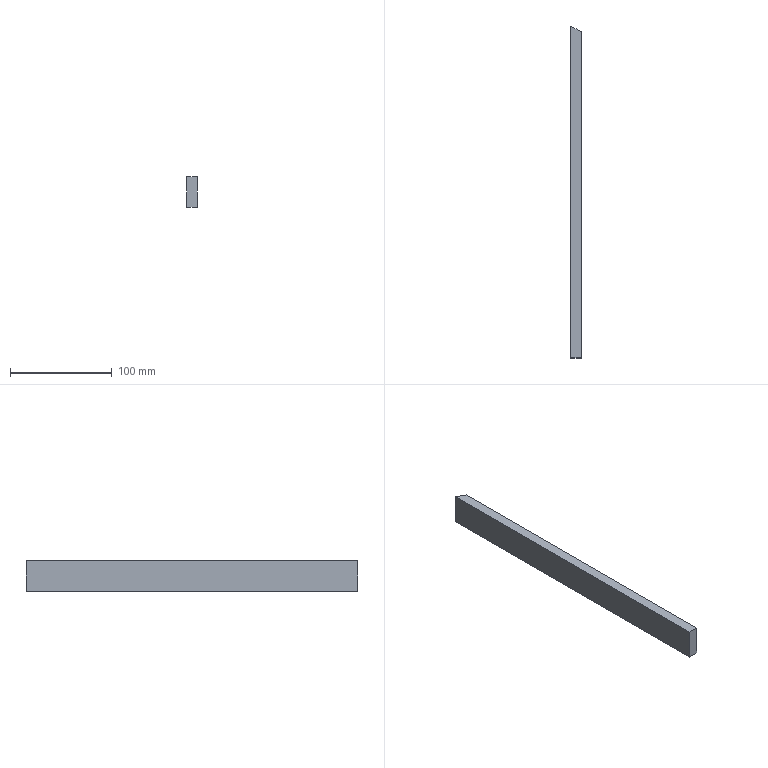Part | NX | features solid 2 | 1 solid | 6 faces | box 10 x 326.105 x 30 mm | volume 96966 mm3 | plane 6
STEP:
#1=CARTESIAN_POINT('',(675.,-588.785,-135.));
#2=VERTEX_POINT('',#1);
#3=CARTESIAN_POINT('',(675.,-588.785,-105.));
#4=VERTEX_POINT('',#3);
#5=CARTESIAN_POINT('',(675.,-588.785,-135.));
#6=DIRECTION('',(0.,0.,-1.));
#7=VECTOR('',#6,1000.);
#8=LINE('',#5,#7);
#9=EDGE_CURVE('',#2,#4,#8,.F.);
#10=ORIENTED_EDGE('',*,*,#9,.F.);
#11=CARTESIAN_POINT('',(675.,-268.453,-135.));
#12=VERTEX_POINT('',#11);
#13=CARTESIAN_POINT('',(675.,-568.785,-135.));
#14=DIRECTION('',(0.,1.,0.));
#15=VECTOR('',#14,1000.);
#16=LINE('',#13,#15);
#17=EDGE_CURVE('',#2,#12,#16,.T.);
#18=ORIENTED_EDGE('',*,*,#17,.T.);
#19=CARTESIAN_POINT('',(675.,-268.453,-105.));
#20=VERTEX_POINT('',#19);
#21=CARTESIAN_POINT('',(675.,-268.453,-135.));
#22=DIRECTION('',(0.,0.,1.));
#23=VECTOR('',#22,1000.);
#24=LINE('',#21,#23);
#25=EDGE_CURVE('',#20,#12,#24,.F.);
#26=ORIENTED_EDGE('',*,*,#25,.F.);
#27=CARTESIAN_POINT('',(675.,-568.785,-105.));
#28=DIRECTION('',(0.,1.,0.));
#29=VECTOR('',#28,1000.);
#30=LINE('',#27,#29);
#31=EDGE_CURVE('',#4,#20,#30,.T.);
#32=ORIENTED_EDGE('',*,*,#31,.F.);
#33=EDGE_LOOP('',(#10,#18,#26,#32));
#34=FACE_BOUND('',#33,.T.);
#35=CARTESIAN_POINT('',(675.,-568.785,-135.));
#36=DIRECTION('',(1.,0.,0.));
#37=DIRECTION('',(0.,0.,-1.));
#38=AXIS2_PLACEMENT_3D('',#35,#36,#37);
#39=PLANE('',#38);
#40=ADVANCED_FACE('',(#34),#39,.T.);
#41=CARTESIAN_POINT('',(665.,-588.785,-105.));
#42=VERTEX_POINT('',#41);
#43=CARTESIAN_POINT('',(675.,-588.785,-105.));
#44=DIRECTION('',(-1.,0.,0.));
#45=VECTOR('',#44,1000.);
#46=LINE('',#43,#45);
#47=EDGE_CURVE('',#42,#4,#46,.F.);
#48=ORIENTED_EDGE('',*,*,#47,.F.);
#49=CARTESIAN_POINT('',(665.,-588.785,-135.));
#50=VERTEX_POINT('',#49);
#51=CARTESIAN_POINT('',(665.,-588.785,-135.));
#52=DIRECTION('',(0.,0.,-1.));
#53=VECTOR('',#52,1000.);
#54=LINE('',#51,#53);
#55=EDGE_CURVE('',#50,#42,#54,.F.);
#56=ORIENTED_EDGE('',*,*,#55,.F.);
#57=CARTESIAN_POINT('',(675.,-588.785,-135.));
#58=DIRECTION('',(-1.,0.,0.));
#59=VECTOR('',#58,1000.);
#60=LINE('',#57,#59);
#61=EDGE_CURVE('',#50,#2,#60,.F.);
#62=ORIENTED_EDGE('',*,*,#61,.T.);
#63=ORIENTED_EDGE('',*,*,#9,.T.);
#64=EDGE_LOOP('',(#48,#56,#62,#63));
#65=FACE_BOUND('',#64,.T.);
#66=CARTESIAN_POINT('',(675.,-588.785,-105.));
#67=DIRECTION('',(0.,-1.,0.));
#68=DIRECTION('',(-1.,0.,0.));
#69=AXIS2_PLACEMENT_3D('',#66,#67,#68);
#70=PLANE('',#69);
#71=ADVANCED_FACE('',(#65),#70,.T.);
#72=CARTESIAN_POINT('',(665.,-262.679,-105.));
#73=VERTEX_POINT('',#72);
#74=CARTESIAN_POINT('',(665.,-262.679,-135.));
#75=VERTEX_POINT('',#74);
#76=CARTESIAN_POINT('',(665.,-262.679,-135.));
#77=DIRECTION('',(0.,0.,1.));
#78=VECTOR('',#77,1000.);
#79=LINE('',#76,#78);
#80=EDGE_CURVE('',#73,#75,#79,.F.);
#81=ORIENTED_EDGE('',*,*,#80,.T.);
#82=CARTESIAN_POINT('',(665.,-568.785,-135.));
#83=DIRECTION('',(0.,-1.,0.));
#84=VECTOR('',#83,1000.);
#85=LINE('',#82,#84);
#86=EDGE_CURVE('',#75,#50,#85,.T.);
#87=ORIENTED_EDGE('',*,*,#86,.T.);
#88=ORIENTED_EDGE('',*,*,#55,.T.);
#89=CARTESIAN_POINT('',(665.,-568.785,-105.));
#90=DIRECTION('',(0.,-1.,0.));
#91=VECTOR('',#90,1000.);
#92=LINE('',#89,#91);
#93=EDGE_CURVE('',#73,#42,#92,.T.);
#94=ORIENTED_EDGE('',*,*,#93,.F.);
#95=EDGE_LOOP('',(#81,#87,#88,#94));
#96=FACE_BOUND('',#95,.T.);
#97=CARTESIAN_POINT('',(665.,-568.785,-135.));
#98=DIRECTION('',(1.,0.,0.));
#99=DIRECTION('',(0.,0.,-1.));
#100=AXIS2_PLACEMENT_3D('',#97,#98,#99);
#101=PLANE('',#100);
#102=ADVANCED_FACE('',(#96),#101,.F.);
#103=CARTESIAN_POINT('',(805.047,-343.536,-135.));
#104=DIRECTION('',(0.866,-0.5,0.));
#105=VECTOR('',#104,1000.);
#106=LINE('',#103,#105);
#107=EDGE_CURVE('',#12,#75,#106,.F.);
#108=ORIENTED_EDGE('',*,*,#107,.T.);
#109=ORIENTED_EDGE('',*,*,#80,.F.);
#110=CARTESIAN_POINT('',(805.047,-343.536,-105.));
#111=DIRECTION('',(0.866,-0.5,0.));
#112=VECTOR('',#111,1000.);
#113=LINE('',#110,#112);
#114=EDGE_CURVE('',#20,#73,#113,.F.);
#115=ORIENTED_EDGE('',*,*,#114,.F.);
#116=ORIENTED_EDGE('',*,*,#25,.T.);
#117=EDGE_LOOP('',(#108,#109,#115,#116));
#118=FACE_BOUND('',#117,.T.);
#119=CARTESIAN_POINT('',(476.795,-154.019,-105.));
#120=DIRECTION('',(0.5,0.866,0.));
#121=DIRECTION('',(0.,0.,-1.));
#122=AXIS2_PLACEMENT_3D('',#119,#120,#121);
#123=PLANE('',#122);
#124=ADVANCED_FACE('',(#118),#123,.T.);
#125=ORIENTED_EDGE('',*,*,#86,.F.);
#126=ORIENTED_EDGE('',*,*,#107,.F.);
#127=ORIENTED_EDGE('',*,*,#17,.F.);
#128=ORIENTED_EDGE('',*,*,#61,.F.);
#129=EDGE_LOOP('',(#125,#126,#127,#128));
#130=FACE_BOUND('',#129,.T.);
#131=CARTESIAN_POINT('',(675.,-568.785,-135.));
#132=DIRECTION('',(0.,0.,-1.));
#133=DIRECTION('',(-1.,0.,0.));
#134=AXIS2_PLACEMENT_3D('',#131,#132,#133);
#135=PLANE('',#134);
#136=ADVANCED_FACE('',(#130),#135,.T.);
#137=ORIENTED_EDGE('',*,*,#114,.T.);
#138=ORIENTED_EDGE('',*,*,#93,.T.);
#139=ORIENTED_EDGE('',*,*,#47,.T.);
#140=ORIENTED_EDGE('',*,*,#31,.T.);
#141=EDGE_LOOP('',(#137,#138,#139,#140));
#142=FACE_BOUND('',#141,.T.);
#143=CARTESIAN_POINT('',(675.,-568.785,-105.));
#144=DIRECTION('',(0.,0.,-1.));
#145=DIRECTION('',(-1.,0.,0.));
#146=AXIS2_PLACEMENT_3D('',#143,#144,#145);
#147=PLANE('',#146);
#148=ADVANCED_FACE('',(#142),#147,.F.);
#149=CLOSED_SHELL('',(#40,#71,#102,#124,#136,#148));
#150=MANIFOLD_SOLID_BREP('',#149);
#151=(LENGTH_UNIT()NAMED_UNIT(*)SI_UNIT(.MILLI.,.METRE.));
#152=UNCERTAINTY_MEASURE_WITH_UNIT(LENGTH_MEASURE(0.00001),#151,'','');
#153=(NAMED_UNIT(*)PLANE_ANGLE_UNIT()SI_UNIT($,.RADIAN.));
#154=(NAMED_UNIT(*)SI_UNIT($,.STERADIAN.)SOLID_ANGLE_UNIT());
#155=(GEOMETRIC_REPRESENTATION_CONTEXT(3)GLOBAL_UNCERTAINTY_ASSIGNED_CONTEXT((#152))GLOBAL_UNIT_ASSIGNED_CONTEXT((#151,#153,#154))REPRESENTATION_CONTEXT('',''));
#156=ADVANCED_BREP_SHAPE_REPRESENTATION('',(#150),#155);